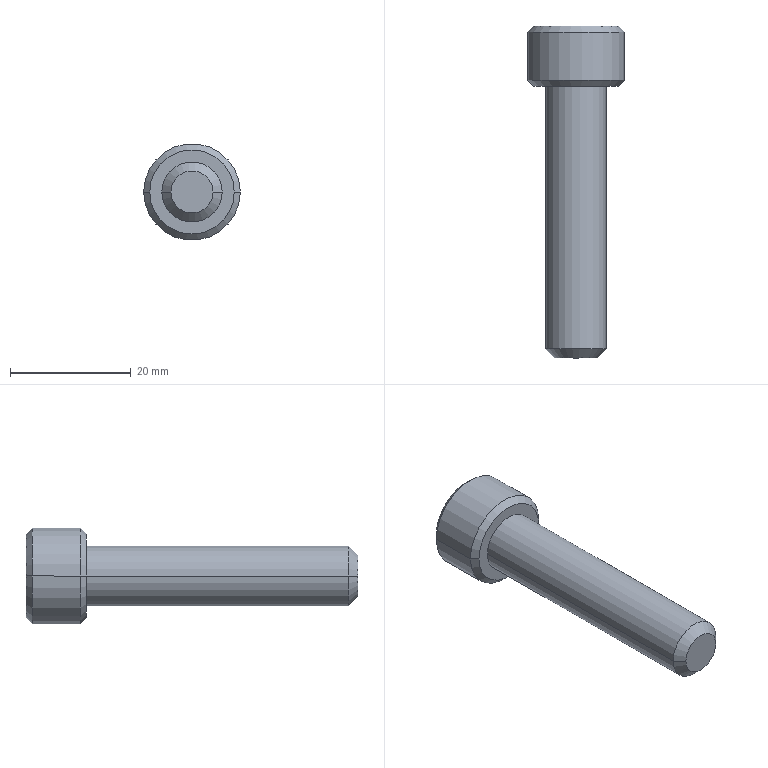Part | STEP file | BB62-M10-45L | 1 solid | 27 faces | box 16 x 55 x 16 mm | volume 5135 mm3 | plane 15 | cone 8 | cylinder 4 | commonest cylinder face diameters 10 x2 16 x2
STEP:
#1=CARTESIAN_POINT('',(0.,2.359,0.));
#2=VERTEX_POINT('',#1);
#3=CARTESIAN_POINT('',(4.575,5.,0.));
#4=VERTEX_POINT('',#3);
#5=CARTESIAN_POINT('',(0.,2.359,0.));
#6=DIRECTION('',(0.866,0.5,0.));
#7=VECTOR('',#6,1000.);
#8=LINE('',#5,#7);
#9=EDGE_CURVE('',#2,#4,#8,.T.);
#10=ORIENTED_EDGE('',*,*,#9,.F.);
#11=CARTESIAN_POINT('',(-4.575,5.,0.));
#12=VERTEX_POINT('',#11);
#13=CARTESIAN_POINT('',(0.,2.359,0.));
#14=DIRECTION('',(-0.866,0.5,0.));
#15=VECTOR('',#14,1000.);
#16=LINE('',#13,#15);
#17=EDGE_CURVE('',#2,#12,#16,.T.);
#18=ORIENTED_EDGE('',*,*,#17,.T.);
#19=CARTESIAN_POINT('',(-3.962,5.,2.288));
#20=VERTEX_POINT('',#19);
#21=CARTESIAN_POINT('',(0.,5.,0.));
#22=DIRECTION('',(0.,-1.,0.));
#23=DIRECTION('',(-1.,0.,0.));
#24=AXIS2_PLACEMENT_3D('',#21,#22,#23);
#25=CIRCLE('',#24,4.575);
#26=EDGE_CURVE('',#20,#12,#25,.T.);
#27=ORIENTED_EDGE('',*,*,#26,.F.);
#28=CARTESIAN_POINT('',(0.,5.,4.575));
#29=VERTEX_POINT('',#28);
#30=CARTESIAN_POINT('',(0.,5.,0.));
#31=DIRECTION('',(0.,-1.,0.));
#32=DIRECTION('',(-1.,0.,0.));
#33=AXIS2_PLACEMENT_3D('',#30,#31,#32);
#34=CIRCLE('',#33,4.575);
#35=EDGE_CURVE('',#29,#20,#34,.T.);
#36=ORIENTED_EDGE('',*,*,#35,.F.);
#37=CARTESIAN_POINT('',(3.962,5.,2.287));
#38=VERTEX_POINT('',#37);
#39=CARTESIAN_POINT('',(0.,5.,0.));
#40=DIRECTION('',(0.,-1.,0.));
#41=DIRECTION('',(-1.,0.,0.));
#42=AXIS2_PLACEMENT_3D('',#39,#40,#41);
#43=CIRCLE('',#42,4.575);
#44=EDGE_CURVE('',#38,#29,#43,.T.);
#45=ORIENTED_EDGE('',*,*,#44,.F.);
#46=CARTESIAN_POINT('',(0.,5.,0.));
#47=DIRECTION('',(0.,-1.,0.));
#48=DIRECTION('',(-1.,0.,0.));
#49=AXIS2_PLACEMENT_3D('',#46,#47,#48);
#50=CIRCLE('',#49,4.575);
#51=EDGE_CURVE('',#4,#38,#50,.T.);
#52=ORIENTED_EDGE('',*,*,#51,.F.);
#53=EDGE_LOOP('',(#10,#18,#27,#36,#45,#52));
#54=FACE_OUTER_BOUND('',#53,.T.);
#55=CARTESIAN_POINT('',(0.,1002.359,0.));
#56=DIRECTION('',(0.,1.,0.));
#57=DIRECTION('',(1.,0.,0.));
#58=AXIS2_PLACEMENT_3D('',#55,#56,#57);
#59=CONICAL_SURFACE('',#58,1732.051,1.047);
#60=ADVANCED_FACE('',(#54),#59,.F.);
#61=CARTESIAN_POINT('',(3.5,-45.,0.));
#62=VERTEX_POINT('',#61);
#63=CARTESIAN_POINT('',(-3.5,-45.,0.));
#64=VERTEX_POINT('',#63);
#65=CARTESIAN_POINT('',(0.,-45.,0.));
#66=DIRECTION('',(0.,1.,0.));
#67=DIRECTION('',(1.,0.,0.));
#68=AXIS2_PLACEMENT_3D('',#65,#66,#67);
#69=CIRCLE('',#68,3.5);
#70=EDGE_CURVE('',#62,#64,#69,.T.);
#71=ORIENTED_EDGE('',*,*,#70,.T.);
#72=CARTESIAN_POINT('',(-5.,-43.5,0.));
#73=VERTEX_POINT('',#72);
#74=CARTESIAN_POINT('',(-3.5,-45.,0.));
#75=DIRECTION('',(-0.7071,0.7071,0.));
#76=VECTOR('',#75,1000.);
#77=LINE('',#74,#76);
#78=EDGE_CURVE('',#64,#73,#77,.T.);
#79=ORIENTED_EDGE('',*,*,#78,.T.);
#80=CARTESIAN_POINT('',(5.,-43.5,0.));
#81=VERTEX_POINT('',#80);
#82=CARTESIAN_POINT('',(0.,-43.5,0.));
#83=DIRECTION('',(0.,-1.,0.));
#84=DIRECTION('',(-1.,0.,0.));
#85=AXIS2_PLACEMENT_3D('',#82,#83,#84);
#86=CIRCLE('',#85,5.);
#87=EDGE_CURVE('',#73,#81,#86,.T.);
#88=ORIENTED_EDGE('',*,*,#87,.T.);
#89=CARTESIAN_POINT('',(3.5,-45.,0.));
#90=DIRECTION('',(0.7071,0.7071,0.));
#91=VECTOR('',#90,1000.);
#92=LINE('',#89,#91);
#93=EDGE_CURVE('',#62,#81,#92,.T.);
#94=ORIENTED_EDGE('',*,*,#93,.F.);
#95=EDGE_LOOP('',(#71,#79,#88,#94));
#96=FACE_OUTER_BOUND('',#95,.T.);
#97=CARTESIAN_POINT('',(0.,-45.,0.));
#98=DIRECTION('',(0.,1.,0.));
#99=DIRECTION('',(1.,0.,0.));
#100=AXIS2_PLACEMENT_3D('',#97,#98,#99);
#101=CONICAL_SURFACE('',#100,3.5,0.7854);
#102=ADVANCED_FACE('',(#96),#101,.T.);
#103=ORIENTED_EDGE('',*,*,#87,.F.);
#104=CARTESIAN_POINT('',(-5.,0.,0.));
#105=VERTEX_POINT('',#104);
#106=CARTESIAN_POINT('',(-5.,-43.5,0.));
#107=DIRECTION('',(0.,1.,0.));
#108=VECTOR('',#107,1000.);
#109=LINE('',#106,#108);
#110=EDGE_CURVE('',#73,#105,#109,.T.);
#111=ORIENTED_EDGE('',*,*,#110,.T.);
#112=CARTESIAN_POINT('',(5.,0.,0.));
#113=VERTEX_POINT('',#112);
#114=CARTESIAN_POINT('',(0.,0.,0.));
#115=DIRECTION('',(0.,-1.,0.));
#116=DIRECTION('',(-1.,0.,0.));
#117=AXIS2_PLACEMENT_3D('',#114,#115,#116);
#118=CIRCLE('',#117,5.);
#119=EDGE_CURVE('',#105,#113,#118,.T.);
#120=ORIENTED_EDGE('',*,*,#119,.T.);
#121=CARTESIAN_POINT('',(5.,-43.5,0.));
#122=DIRECTION('',(0.,1.,0.));
#123=VECTOR('',#122,1000.);
#124=LINE('',#121,#123);
#125=EDGE_CURVE('',#81,#113,#124,.T.);
#126=ORIENTED_EDGE('',*,*,#125,.F.);
#127=EDGE_LOOP('',(#103,#111,#120,#126));
#128=FACE_OUTER_BOUND('',#127,.T.);
#129=CARTESIAN_POINT('',(0.,-43.5,0.));
#130=DIRECTION('',(0.,1.,0.));
#131=DIRECTION('',(1.,0.,0.));
#132=AXIS2_PLACEMENT_3D('',#129,#130,#131);
#133=CYLINDRICAL_SURFACE('',#132,5.);
#134=ADVANCED_FACE('',(#128),#133,.T.);
#135=CARTESIAN_POINT('',(-7.,10.,0.));
#136=VERTEX_POINT('',#135);
#137=CARTESIAN_POINT('',(7.,10.,0.));
#138=VERTEX_POINT('',#137);
#139=CARTESIAN_POINT('',(0.,10.,0.));
#140=DIRECTION('',(0.,-1.,0.));
#141=DIRECTION('',(-1.,0.,0.));
#142=AXIS2_PLACEMENT_3D('',#139,#140,#141);
#143=CIRCLE('',#142,7.);
#144=EDGE_CURVE('',#136,#138,#143,.T.);
#145=ORIENTED_EDGE('',*,*,#144,.T.);
#146=CARTESIAN_POINT('',(8.,9.,0.));
#147=VERTEX_POINT('',#146);
#148=CARTESIAN_POINT('',(8.,9.,0.));
#149=DIRECTION('',(0.7071,-0.7071,0.));
#150=VECTOR('',#149,1000.);
#151=LINE('',#148,#150);
#152=EDGE_CURVE('',#138,#147,#151,.T.);
#153=ORIENTED_EDGE('',*,*,#152,.T.);
#154=CARTESIAN_POINT('',(-8.,9.,0.));
#155=VERTEX_POINT('',#154);
#156=CARTESIAN_POINT('',(0.,9.,0.));
#157=DIRECTION('',(0.,-1.,0.));
#158=DIRECTION('',(-1.,0.,0.));
#159=AXIS2_PLACEMENT_3D('',#156,#157,#158);
#160=CIRCLE('',#159,8.);
#161=EDGE_CURVE('',#155,#147,#160,.T.);
#162=ORIENTED_EDGE('',*,*,#161,.F.);
#163=CARTESIAN_POINT('',(-8.,9.,0.));
#164=DIRECTION('',(-0.7071,-0.7071,0.));
#165=VECTOR('',#164,1000.);
#166=LINE('',#163,#165);
#167=EDGE_CURVE('',#136,#155,#166,.T.);
#168=ORIENTED_EDGE('',*,*,#167,.F.);
#169=EDGE_LOOP('',(#145,#153,#162,#168));
#170=FACE_OUTER_BOUND('',#169,.T.);
#171=CARTESIAN_POINT('',(0.,9.,0.));
#172=DIRECTION('',(0.,-1.,0.));
#173=DIRECTION('',(-1.,0.,0.));
#174=AXIS2_PLACEMENT_3D('',#171,#172,#173);
#175=CONICAL_SURFACE('',#174,8.,0.7854);
#176=ADVANCED_FACE('',(#170),#175,.T.);
#177=ORIENTED_EDGE('',*,*,#161,.T.);
#178=CARTESIAN_POINT('',(8.,1.,0.));
#179=VERTEX_POINT('',#178);
#180=CARTESIAN_POINT('',(8.,1.62,0.));
#181=DIRECTION('',(0.,-1.,0.));
#182=VECTOR('',#181,1000.);
#183=LINE('',#180,#182);
#184=EDGE_CURVE('',#147,#179,#183,.T.);
#185=ORIENTED_EDGE('',*,*,#184,.T.);
#186=CARTESIAN_POINT('',(-8.,1.,0.));
#187=VERTEX_POINT('',#186);
#188=CARTESIAN_POINT('',(0.,1.,0.));
#189=DIRECTION('',(0.,-1.,0.));
#190=DIRECTION('',(-1.,0.,0.));
#191=AXIS2_PLACEMENT_3D('',#188,#189,#190);
#192=CIRCLE('',#191,8.);
#193=EDGE_CURVE('',#187,#179,#192,.T.);
#194=ORIENTED_EDGE('',*,*,#193,.F.);
#195=CARTESIAN_POINT('',(-8.,1.62,0.));
#196=DIRECTION('',(0.,-1.,0.));
#197=VECTOR('',#196,1000.);
#198=LINE('',#195,#197);
#199=EDGE_CURVE('',#155,#187,#198,.T.);
#200=ORIENTED_EDGE('',*,*,#199,.F.);
#201=EDGE_LOOP('',(#177,#185,#194,#200));
#202=FACE_OUTER_BOUND('',#201,.T.);
#203=CARTESIAN_POINT('',(0.,1.62,0.));
#204=DIRECTION('',(0.,-1.,0.));
#205=DIRECTION('',(-1.,0.,0.));
#206=AXIS2_PLACEMENT_3D('',#203,#204,#205);
#207=CYLINDRICAL_SURFACE('',#206,8.);
#208=ADVANCED_FACE('',(#202),#207,.T.);
#209=CARTESIAN_POINT('',(-7.,0.,0.));
#210=VERTEX_POINT('',#209);
#211=CARTESIAN_POINT('',(7.,0.,0.));
#212=VERTEX_POINT('',#211);
#213=CARTESIAN_POINT('',(0.,0.,0.));
#214=DIRECTION('',(0.,-1.,0.));
#215=DIRECTION('',(-1.,0.,0.));
#216=AXIS2_PLACEMENT_3D('',#213,#214,#215);
#217=CIRCLE('',#216,7.);
#218=EDGE_CURVE('',#210,#212,#217,.T.);
#219=ORIENTED_EDGE('',*,*,#218,.F.);
#220=CARTESIAN_POINT('',(-7.,0.,0.));
#221=DIRECTION('',(-0.7071,0.7071,0.));
#222=VECTOR('',#221,1000.);
#223=LINE('',#220,#222);
#224=EDGE_CURVE('',#210,#187,#223,.T.);
#225=ORIENTED_EDGE('',*,*,#224,.T.);
#226=ORIENTED_EDGE('',*,*,#193,.T.);
#227=CARTESIAN_POINT('',(7.,0.,0.));
#228=DIRECTION('',(0.7071,0.7071,0.));
#229=VECTOR('',#228,1000.);
#230=LINE('',#227,#229);
#231=EDGE_CURVE('',#212,#179,#230,.T.);
#232=ORIENTED_EDGE('',*,*,#231,.F.);
#233=EDGE_LOOP('',(#219,#225,#226,#232));
#234=FACE_OUTER_BOUND('',#233,.T.);
#235=CARTESIAN_POINT('',(0.,0.,0.));
#236=DIRECTION('',(0.,1.,0.));
#237=DIRECTION('',(1.,0.,0.));
#238=AXIS2_PLACEMENT_3D('',#235,#236,#237);
#239=CONICAL_SURFACE('',#238,7.,0.7854);
#240=ADVANCED_FACE('',(#234),#239,.T.);
#241=ORIENTED_EDGE('',*,*,#144,.F.);
#242=CARTESIAN_POINT('',(0.,10.,0.));
#243=DIRECTION('',(0.,-1.,0.));
#244=DIRECTION('',(-1.,0.,0.));
#245=AXIS2_PLACEMENT_3D('',#242,#243,#244);
#246=CIRCLE('',#245,7.);
#247=EDGE_CURVE('',#138,#136,#246,.T.);
#248=ORIENTED_EDGE('',*,*,#247,.F.);
#249=EDGE_LOOP('',(#241,#248));
#250=FACE_OUTER_BOUND('',#249,.T.);
#251=CARTESIAN_POINT('',(0.,10.,-4.575));
#252=VERTEX_POINT('',#251);
#253=CARTESIAN_POINT('',(-3.962,10.,-2.287));
#254=VERTEX_POINT('',#253);
#255=CARTESIAN_POINT('',(0.,10.,-4.575));
#256=DIRECTION('',(-0.866,0.,0.5));
#257=VECTOR('',#256,1000.);
#258=LINE('',#255,#257);
#259=EDGE_CURVE('',#252,#254,#258,.T.);
#260=ORIENTED_EDGE('',*,*,#259,.F.);
#261=CARTESIAN_POINT('',(3.962,10.,-2.287));
#262=VERTEX_POINT('',#261);
#263=CARTESIAN_POINT('',(3.962,10.,-2.287));
#264=DIRECTION('',(-0.866,0.,-0.5));
#265=VECTOR('',#264,1000.);
#266=LINE('',#263,#265);
#267=EDGE_CURVE('',#262,#252,#266,.T.);
#268=ORIENTED_EDGE('',*,*,#267,.F.);
#269=CARTESIAN_POINT('',(3.962,10.,2.288));
#270=VERTEX_POINT('',#269);
#271=CARTESIAN_POINT('',(3.962,10.,2.288));
#272=DIRECTION('',(0.,0.,-1.));
#273=VECTOR('',#272,1000.);
#274=LINE('',#271,#273);
#275=EDGE_CURVE('',#270,#262,#274,.T.);
#276=ORIENTED_EDGE('',*,*,#275,.F.);
#277=CARTESIAN_POINT('',(0.,10.,4.575));
#278=VERTEX_POINT('',#277);
#279=CARTESIAN_POINT('',(0.,10.,4.575));
#280=DIRECTION('',(0.866,0.,-0.5));
#281=VECTOR('',#280,1000.);
#282=LINE('',#279,#281);
#283=EDGE_CURVE('',#278,#270,#282,.T.);
#284=ORIENTED_EDGE('',*,*,#283,.F.);
#285=CARTESIAN_POINT('',(-3.962,10.,2.288));
#286=VERTEX_POINT('',#285);
#287=CARTESIAN_POINT('',(-3.962,10.,2.288));
#288=DIRECTION('',(0.866,0.,0.5));
#289=VECTOR('',#288,1000.);
#290=LINE('',#287,#289);
#291=EDGE_CURVE('',#286,#278,#290,.T.);
#292=ORIENTED_EDGE('',*,*,#291,.F.);
#293=CARTESIAN_POINT('',(-3.962,10.,-2.287));
#294=DIRECTION('',(0.,0.,1.));
#295=VECTOR('',#294,1000.);
#296=LINE('',#293,#295);
#297=EDGE_CURVE('',#254,#286,#296,.T.);
#298=ORIENTED_EDGE('',*,*,#297,.F.);
#299=EDGE_LOOP('',(#260,#268,#276,#284,#292,#298));
#300=FACE_BOUND('',#299,.T.);
#301=CARTESIAN_POINT('',(7.,10.,0.));
#302=DIRECTION('',(0.,1.,0.));
#303=DIRECTION('',(1.,0.,0.));
#304=AXIS2_PLACEMENT_3D('',#301,#302,#303);
#305=PLANE('',#304);
#306=ADVANCED_FACE('',(#250,#300),#305,.T.);
#307=CARTESIAN_POINT('',(0.,0.,0.));
#308=DIRECTION('',(0.,-1.,0.));
#309=DIRECTION('',(-1.,0.,0.));
#310=AXIS2_PLACEMENT_3D('',#307,#308,#309);
#311=CIRCLE('',#310,5.);
#312=EDGE_CURVE('',#113,#105,#311,.T.);
#313=ORIENTED_EDGE('',*,*,#312,.F.);
#314=ORIENTED_EDGE('',*,*,#119,.F.);
#315=EDGE_LOOP('',(#313,#314));
#316=FACE_BOUND('',#315,.T.);
#317=CARTESIAN_POINT('',(0.,0.,0.));
#318=DIRECTION('',(0.,-1.,0.));
#319=DIRECTION('',(-1.,0.,0.));
#320=AXIS2_PLACEMENT_3D('',#317,#318,#319);
#321=CIRCLE('',#320,7.);
#322=EDGE_CURVE('',#212,#210,#321,.T.);
#323=ORIENTED_EDGE('',*,*,#322,.T.);
#324=ORIENTED_EDGE('',*,*,#218,.T.);
#325=EDGE_LOOP('',(#323,#324));
#326=FACE_OUTER_BOUND('',#325,.T.);
#327=CARTESIAN_POINT('',(0.,0.,0.));
#328=DIRECTION('',(0.,-1.,0.));
#329=DIRECTION('',(-1.,0.,0.));
#330=AXIS2_PLACEMENT_3D('',#327,#328,#329);
#331=PLANE('',#330);
#332=ADVANCED_FACE('',(#316,#326),#331,.T.);
#333=ORIENTED_EDGE('',*,*,#224,.F.);
#334=ORIENTED_EDGE('',*,*,#322,.F.);
#335=ORIENTED_EDGE('',*,*,#231,.T.);
#336=CARTESIAN_POINT('',(0.,1.,0.));
#337=DIRECTION('',(0.,-1.,0.));
#338=DIRECTION('',(-1.,0.,0.));
#339=AXIS2_PLACEMENT_3D('',#336,#337,#338);
#340=CIRCLE('',#339,8.);
#341=EDGE_CURVE('',#179,#187,#340,.T.);
#342=ORIENTED_EDGE('',*,*,#341,.T.);
#343=EDGE_LOOP('',(#333,#334,#335,#342));
#344=FACE_OUTER_BOUND('',#343,.T.);
#345=CARTESIAN_POINT('',(0.,0.,0.));
#346=DIRECTION('',(0.,1.,0.));
#347=DIRECTION('',(1.,0.,0.));
#348=AXIS2_PLACEMENT_3D('',#345,#346,#347);
#349=CONICAL_SURFACE('',#348,7.,0.7854);
#350=ADVANCED_FACE('',(#344),#349,.T.);
#351=ORIENTED_EDGE('',*,*,#184,.F.);
#352=CARTESIAN_POINT('',(0.,9.,0.));
#353=DIRECTION('',(0.,-1.,0.));
#354=DIRECTION('',(-1.,0.,0.));
#355=AXIS2_PLACEMENT_3D('',#352,#353,#354);
#356=CIRCLE('',#355,8.);
#357=EDGE_CURVE('',#147,#155,#356,.T.);
#358=ORIENTED_EDGE('',*,*,#357,.T.);
#359=ORIENTED_EDGE('',*,*,#199,.T.);
#360=ORIENTED_EDGE('',*,*,#341,.F.);
#361=EDGE_LOOP('',(#351,#358,#359,#360));
#362=FACE_OUTER_BOUND('',#361,.T.);
#363=CARTESIAN_POINT('',(0.,1.62,0.));
#364=DIRECTION('',(0.,-1.,0.));
#365=DIRECTION('',(-1.,0.,0.));
#366=AXIS2_PLACEMENT_3D('',#363,#364,#365);
#367=CYLINDRICAL_SURFACE('',#366,8.);
#368=ADVANCED_FACE('',(#362),#367,.T.);
#369=ORIENTED_EDGE('',*,*,#152,.F.);
#370=ORIENTED_EDGE('',*,*,#247,.T.);
#371=ORIENTED_EDGE('',*,*,#167,.T.);
#372=ORIENTED_EDGE('',*,*,#357,.F.);
#373=EDGE_LOOP('',(#369,#370,#371,#372));
#374=FACE_OUTER_BOUND('',#373,.T.);
#375=CARTESIAN_POINT('',(0.,9.,0.));
#376=DIRECTION('',(0.,-1.,0.));
#377=DIRECTION('',(-1.,0.,0.));
#378=AXIS2_PLACEMENT_3D('',#375,#376,#377);
#379=CONICAL_SURFACE('',#378,8.,0.7854);
#380=ADVANCED_FACE('',(#374),#379,.T.);
#381=ORIENTED_EDGE('',*,*,#110,.F.);
#382=CARTESIAN_POINT('',(0.,-43.5,0.));
#383=DIRECTION('',(0.,-1.,0.));
#384=DIRECTION('',(-1.,0.,0.));
#385=AXIS2_PLACEMENT_3D('',#382,#383,#384);
#386=CIRCLE('',#385,5.);
#387=EDGE_CURVE('',#81,#73,#386,.T.);
#388=ORIENTED_EDGE('',*,*,#387,.F.);
#389=ORIENTED_EDGE('',*,*,#125,.T.);
#390=ORIENTED_EDGE('',*,*,#312,.T.);
#391=EDGE_LOOP('',(#381,#388,#389,#390));
#392=FACE_OUTER_BOUND('',#391,.T.);
#393=CARTESIAN_POINT('',(0.,-43.5,0.));
#394=DIRECTION('',(0.,1.,0.));
#395=DIRECTION('',(1.,0.,0.));
#396=AXIS2_PLACEMENT_3D('',#393,#394,#395);
#397=CYLINDRICAL_SURFACE('',#396,5.);
#398=ADVANCED_FACE('',(#392),#397,.T.);
#399=ORIENTED_EDGE('',*,*,#70,.F.);
#400=CARTESIAN_POINT('',(0.,-45.,0.));
#401=DIRECTION('',(0.,1.,0.));
#402=DIRECTION('',(1.,0.,0.));
#403=AXIS2_PLACEMENT_3D('',#400,#401,#402);
#404=CIRCLE('',#403,3.5);
#405=EDGE_CURVE('',#64,#62,#404,.T.);
#406=ORIENTED_EDGE('',*,*,#405,.F.);
#407=EDGE_LOOP('',(#399,#406));
#408=FACE_OUTER_BOUND('',#407,.T.);
#409=CARTESIAN_POINT('',(0.,-45.,0.));
#410=DIRECTION('',(0.,-1.,0.));
#411=DIRECTION('',(-1.,0.,0.));
#412=AXIS2_PLACEMENT_3D('',#409,#410,#411);
#413=PLANE('',#412);
#414=ADVANCED_FACE('',(#408),#413,.T.);
#415=ORIENTED_EDGE('',*,*,#78,.F.);
#416=ORIENTED_EDGE('',*,*,#405,.T.);
#417=ORIENTED_EDGE('',*,*,#93,.T.);
#418=ORIENTED_EDGE('',*,*,#387,.T.);
#419=EDGE_LOOP('',(#415,#416,#417,#418));
#420=FACE_OUTER_BOUND('',#419,.T.);
#421=CARTESIAN_POINT('',(0.,-45.,0.));
#422=DIRECTION('',(0.,1.,0.));
#423=DIRECTION('',(1.,0.,0.));
#424=AXIS2_PLACEMENT_3D('',#421,#422,#423);
#425=CONICAL_SURFACE('',#424,3.5,0.7854);
#426=ADVANCED_FACE('',(#420),#425,.T.);
#427=CARTESIAN_POINT('',(3.962,5.,-2.288));
#428=VERTEX_POINT('',#427);
#429=CARTESIAN_POINT('',(0.,5.,-4.575));
#430=VERTEX_POINT('',#429);
#431=CARTESIAN_POINT('',(3.962,5.,-2.288));
#432=DIRECTION('',(-0.866,0.,-0.5));
#433=VECTOR('',#432,1000.);
#434=LINE('',#431,#433);
#435=EDGE_CURVE('',#428,#430,#434,.T.);
#436=ORIENTED_EDGE('',*,*,#435,.F.);
#437=CARTESIAN_POINT('',(3.962,10.,-2.287));
#438=DIRECTION('',(0.,-1.,0.));
#439=VECTOR('',#438,1000.);
#440=LINE('',#437,#439);
#441=EDGE_CURVE('',#262,#428,#440,.T.);
#442=ORIENTED_EDGE('',*,*,#441,.F.);
#443=ORIENTED_EDGE('',*,*,#267,.T.);
#444=CARTESIAN_POINT('',(0.,10.,-4.575));
#445=DIRECTION('',(0.,-1.,0.));
#446=VECTOR('',#445,1000.);
#447=LINE('',#444,#446);
#448=EDGE_CURVE('',#252,#430,#447,.T.);
#449=ORIENTED_EDGE('',*,*,#448,.T.);
#450=EDGE_LOOP('',(#436,#442,#443,#449));
#451=FACE_OUTER_BOUND('',#450,.T.);
#452=CARTESIAN_POINT('',(3.962,10.,-2.287));
#453=DIRECTION('',(-0.5,0.,0.866));
#454=DIRECTION('',(0.866,0.,0.5));
#455=AXIS2_PLACEMENT_3D('',#452,#453,#454);
#456=PLANE('',#455);
#457=ADVANCED_FACE('',(#451),#456,.T.);
#458=CARTESIAN_POINT('',(-3.962,5.,-2.288));
#459=VERTEX_POINT('',#458);
#460=CARTESIAN_POINT('',(0.,5.,-4.575));
#461=DIRECTION('',(-0.866,0.,0.5));
#462=VECTOR('',#461,1000.);
#463=LINE('',#460,#462);
#464=EDGE_CURVE('',#430,#459,#463,.T.);
#465=ORIENTED_EDGE('',*,*,#464,.F.);
#466=ORIENTED_EDGE('',*,*,#448,.F.);
#467=ORIENTED_EDGE('',*,*,#259,.T.);
#468=CARTESIAN_POINT('',(-3.962,10.,-2.287));
#469=DIRECTION('',(0.,-1.,0.));
#470=VECTOR('',#469,1000.);
#471=LINE('',#468,#470);
#472=EDGE_CURVE('',#254,#459,#471,.T.);
#473=ORIENTED_EDGE('',*,*,#472,.T.);
#474=EDGE_LOOP('',(#465,#466,#467,#473));
#475=FACE_OUTER_BOUND('',#474,.T.);
#476=CARTESIAN_POINT('',(0.,10.,-4.575));
#477=DIRECTION('',(0.5,0.,0.866));
#478=DIRECTION('',(0.866,0.,-0.5));
#479=AXIS2_PLACEMENT_3D('',#476,#477,#478);
#480=PLANE('',#479);
#481=ADVANCED_FACE('',(#475),#480,.T.);
#482=CARTESIAN_POINT('',(-3.962,5.,-2.288));
#483=DIRECTION('',(0.,0.,1.));
#484=VECTOR('',#483,1000.);
#485=LINE('',#482,#484);
#486=EDGE_CURVE('',#459,#20,#485,.T.);
#487=ORIENTED_EDGE('',*,*,#486,.F.);
#488=ORIENTED_EDGE('',*,*,#472,.F.);
#489=ORIENTED_EDGE('',*,*,#297,.T.);
#490=CARTESIAN_POINT('',(-3.962,10.,2.288));
#491=DIRECTION('',(0.,-1.,0.));
#492=VECTOR('',#491,1000.);
#493=LINE('',#490,#492);
#494=EDGE_CURVE('',#286,#20,#493,.T.);
#495=ORIENTED_EDGE('',*,*,#494,.T.);
#496=EDGE_LOOP('',(#487,#488,#489,#495));
#497=FACE_OUTER_BOUND('',#496,.T.);
#498=CARTESIAN_POINT('',(-3.962,10.,-2.287));
#499=DIRECTION('',(1.,0.,0.));
#500=DIRECTION('',(0.,0.,-1.));
#501=AXIS2_PLACEMENT_3D('',#498,#499,#500);
#502=PLANE('',#501);
#503=ADVANCED_FACE('',(#497),#502,.T.);
#504=CARTESIAN_POINT('',(-3.962,5.,2.287));
#505=DIRECTION('',(0.866,0.,0.5));
#506=VECTOR('',#505,1000.);
#507=LINE('',#504,#506);
#508=EDGE_CURVE('',#20,#29,#507,.T.);
#509=ORIENTED_EDGE('',*,*,#508,.F.);
#510=ORIENTED_EDGE('',*,*,#494,.F.);
#511=ORIENTED_EDGE('',*,*,#291,.T.);
#512=CARTESIAN_POINT('',(0.,10.,4.575));
#513=DIRECTION('',(0.,-1.,0.));
#514=VECTOR('',#513,1000.);
#515=LINE('',#512,#514);
#516=EDGE_CURVE('',#278,#29,#515,.T.);
#517=ORIENTED_EDGE('',*,*,#516,.T.);
#518=EDGE_LOOP('',(#509,#510,#511,#517));
#519=FACE_OUTER_BOUND('',#518,.T.);
#520=CARTESIAN_POINT('',(-3.962,10.,2.288));
#521=DIRECTION('',(0.5,0.,-0.866));
#522=DIRECTION('',(-0.866,0.,-0.5));
#523=AXIS2_PLACEMENT_3D('',#520,#521,#522);
#524=PLANE('',#523);
#525=ADVANCED_FACE('',(#519),#524,.T.);
#526=CARTESIAN_POINT('',(0.,5.,4.575));
#527=DIRECTION('',(0.866,0.,-0.5));
#528=VECTOR('',#527,1000.);
#529=LINE('',#526,#528);
#530=EDGE_CURVE('',#29,#38,#529,.T.);
#531=ORIENTED_EDGE('',*,*,#530,.F.);
#532=ORIENTED_EDGE('',*,*,#516,.F.);
#533=ORIENTED_EDGE('',*,*,#283,.T.);
#534=CARTESIAN_POINT('',(3.962,10.,2.288));
#535=DIRECTION('',(0.,-1.,0.));
#536=VECTOR('',#535,1000.);
#537=LINE('',#534,#536);
#538=EDGE_CURVE('',#270,#38,#537,.T.);
#539=ORIENTED_EDGE('',*,*,#538,.T.);
#540=EDGE_LOOP('',(#531,#532,#533,#539));
#541=FACE_OUTER_BOUND('',#540,.T.);
#542=CARTESIAN_POINT('',(0.,10.,4.575));
#543=DIRECTION('',(-0.5,0.,-0.866));
#544=DIRECTION('',(-0.866,0.,0.5));
#545=AXIS2_PLACEMENT_3D('',#542,#543,#544);
#546=PLANE('',#545);
#547=ADVANCED_FACE('',(#541),#546,.T.);
#548=CARTESIAN_POINT('',(3.962,5.,2.287));
#549=DIRECTION('',(0.,0.,-1.));
#550=VECTOR('',#549,1000.);
#551=LINE('',#548,#550);
#552=EDGE_CURVE('',#38,#428,#551,.T.);
#553=ORIENTED_EDGE('',*,*,#552,.F.);
#554=ORIENTED_EDGE('',*,*,#538,.F.);
#555=ORIENTED_EDGE('',*,*,#275,.T.);
#556=ORIENTED_EDGE('',*,*,#441,.T.);
#557=EDGE_LOOP('',(#553,#554,#555,#556));
#558=FACE_OUTER_BOUND('',#557,.T.);
#559=CARTESIAN_POINT('',(3.962,10.,2.288));
#560=DIRECTION('',(-1.,0.,0.));
#561=DIRECTION('',(0.,0.,1.));
#562=AXIS2_PLACEMENT_3D('',#559,#560,#561);
#563=PLANE('',#562);
#564=ADVANCED_FACE('',(#558),#563,.T.);
#565=ORIENTED_EDGE('',*,*,#435,.T.);
#566=CARTESIAN_POINT('',(0.,5.,0.));
#567=DIRECTION('',(0.,-1.,0.));
#568=DIRECTION('',(-1.,0.,0.));
#569=AXIS2_PLACEMENT_3D('',#566,#567,#568);
#570=CIRCLE('',#569,4.575);
#571=EDGE_CURVE('',#430,#428,#570,.T.);
#572=ORIENTED_EDGE('',*,*,#571,.T.);
#573=EDGE_LOOP('',(#565,#572));
#574=FACE_OUTER_BOUND('',#573,.T.);
#575=CARTESIAN_POINT('',(0.,5.,0.));
#576=DIRECTION('',(0.,1.,0.));
#577=DIRECTION('',(1.,0.,0.));
#578=AXIS2_PLACEMENT_3D('',#575,#576,#577);
#579=PLANE('',#578);
#580=ADVANCED_FACE('',(#574),#579,.F.);
#581=ORIENTED_EDGE('',*,*,#552,.T.);
#582=CARTESIAN_POINT('',(0.,5.,0.));
#583=DIRECTION('',(0.,-1.,0.));
#584=DIRECTION('',(-1.,0.,0.));
#585=AXIS2_PLACEMENT_3D('',#582,#583,#584);
#586=CIRCLE('',#585,4.575);
#587=EDGE_CURVE('',#428,#4,#586,.T.);
#588=ORIENTED_EDGE('',*,*,#587,.T.);
#589=ORIENTED_EDGE('',*,*,#51,.T.);
#590=EDGE_LOOP('',(#581,#588,#589));
#591=FACE_OUTER_BOUND('',#590,.T.);
#592=CARTESIAN_POINT('',(0.,5.,0.));
#593=DIRECTION('',(0.,1.,0.));
#594=DIRECTION('',(1.,0.,0.));
#595=AXIS2_PLACEMENT_3D('',#592,#593,#594);
#596=PLANE('',#595);
#597=ADVANCED_FACE('',(#591),#596,.F.);
#598=ORIENTED_EDGE('',*,*,#530,.T.);
#599=ORIENTED_EDGE('',*,*,#44,.T.);
#600=EDGE_LOOP('',(#598,#599));
#601=FACE_OUTER_BOUND('',#600,.T.);
#602=CARTESIAN_POINT('',(0.,5.,0.));
#603=DIRECTION('',(0.,1.,0.));
#604=DIRECTION('',(1.,0.,0.));
#605=AXIS2_PLACEMENT_3D('',#602,#603,#604);
#606=PLANE('',#605);
#607=ADVANCED_FACE('',(#601),#606,.F.);
#608=ORIENTED_EDGE('',*,*,#508,.T.);
#609=ORIENTED_EDGE('',*,*,#35,.T.);
#610=EDGE_LOOP('',(#608,#609));
#611=FACE_OUTER_BOUND('',#610,.T.);
#612=CARTESIAN_POINT('',(0.,5.,0.));
#613=DIRECTION('',(0.,1.,0.));
#614=DIRECTION('',(1.,0.,0.));
#615=AXIS2_PLACEMENT_3D('',#612,#613,#614);
#616=PLANE('',#615);
#617=ADVANCED_FACE('',(#611),#616,.F.);
#618=ORIENTED_EDGE('',*,*,#486,.T.);
#619=ORIENTED_EDGE('',*,*,#26,.T.);
#620=CARTESIAN_POINT('',(0.,5.,0.));
#621=DIRECTION('',(0.,-1.,0.));
#622=DIRECTION('',(-1.,0.,0.));
#623=AXIS2_PLACEMENT_3D('',#620,#621,#622);
#624=CIRCLE('',#623,4.575);
#625=EDGE_CURVE('',#12,#459,#624,.T.);
#626=ORIENTED_EDGE('',*,*,#625,.T.);
#627=EDGE_LOOP('',(#618,#619,#626));
#628=FACE_OUTER_BOUND('',#627,.T.);
#629=CARTESIAN_POINT('',(0.,5.,0.));
#630=DIRECTION('',(0.,1.,0.));
#631=DIRECTION('',(1.,0.,0.));
#632=AXIS2_PLACEMENT_3D('',#629,#630,#631);
#633=PLANE('',#632);
#634=ADVANCED_FACE('',(#628),#633,.F.);
#635=ORIENTED_EDGE('',*,*,#464,.T.);
#636=CARTESIAN_POINT('',(0.,5.,0.));
#637=DIRECTION('',(0.,-1.,0.));
#638=DIRECTION('',(-1.,0.,0.));
#639=AXIS2_PLACEMENT_3D('',#636,#637,#638);
#640=CIRCLE('',#639,4.575);
#641=EDGE_CURVE('',#459,#430,#640,.T.);
#642=ORIENTED_EDGE('',*,*,#641,.T.);
#643=EDGE_LOOP('',(#635,#642));
#644=FACE_OUTER_BOUND('',#643,.T.);
#645=CARTESIAN_POINT('',(0.,5.,0.));
#646=DIRECTION('',(0.,1.,0.));
#647=DIRECTION('',(1.,0.,0.));
#648=AXIS2_PLACEMENT_3D('',#645,#646,#647);
#649=PLANE('',#648);
#650=ADVANCED_FACE('',(#644),#649,.F.);
#651=ORIENTED_EDGE('',*,*,#17,.F.);
#652=ORIENTED_EDGE('',*,*,#9,.T.);
#653=ORIENTED_EDGE('',*,*,#587,.F.);
#654=ORIENTED_EDGE('',*,*,#571,.F.);
#655=ORIENTED_EDGE('',*,*,#641,.F.);
#656=ORIENTED_EDGE('',*,*,#625,.F.);
#657=EDGE_LOOP('',(#651,#652,#653,#654,#655,#656));
#658=FACE_OUTER_BOUND('',#657,.T.);
#659=CARTESIAN_POINT('',(0.,1002.359,0.));
#660=DIRECTION('',(0.,1.,0.));
#661=DIRECTION('',(1.,0.,0.));
#662=AXIS2_PLACEMENT_3D('',#659,#660,#661);
#663=CONICAL_SURFACE('',#662,1732.051,1.047);
#664=ADVANCED_FACE('',(#658),#663,.F.);
#665=CLOSED_SHELL('',(#60,#102,#134,#176,#208,#240,#306,#332,#350,#368,#380,#398,#414,#426,#457,#481,#503,#525,#547,#564,#580,#597,#607,#617,#634,#650,#664));
#666=MANIFOLD_SOLID_BREP('',#665);
#667=CARTESIAN_POINT('',(0.,0.,0.));
#668=DIRECTION('',(0.,0.,1.));
#669=DIRECTION('',(1.,0.,0.));
#670=AXIS2_PLACEMENT_3D('',#667,#668,#669);
#671=(LENGTH_UNIT()NAMED_UNIT(*)SI_UNIT(.MILLI.,.METRE.));
#672=UNCERTAINTY_MEASURE_WITH_UNIT(LENGTH_MEASURE(0.00001),#671,'','');
#673=(NAMED_UNIT(*)PLANE_ANGLE_UNIT()SI_UNIT($,.RADIAN.));
#674=(NAMED_UNIT(*)SI_UNIT($,.STERADIAN.)SOLID_ANGLE_UNIT());
#675=(GEOMETRIC_REPRESENTATION_CONTEXT(3)GLOBAL_UNCERTAINTY_ASSIGNED_CONTEXT((#672))GLOBAL_UNIT_ASSIGNED_CONTEXT((#671,#673,#674))REPRESENTATION_CONTEXT('',''));
#676=ADVANCED_BREP_SHAPE_REPRESENTATION('',(#666,#670),#675);